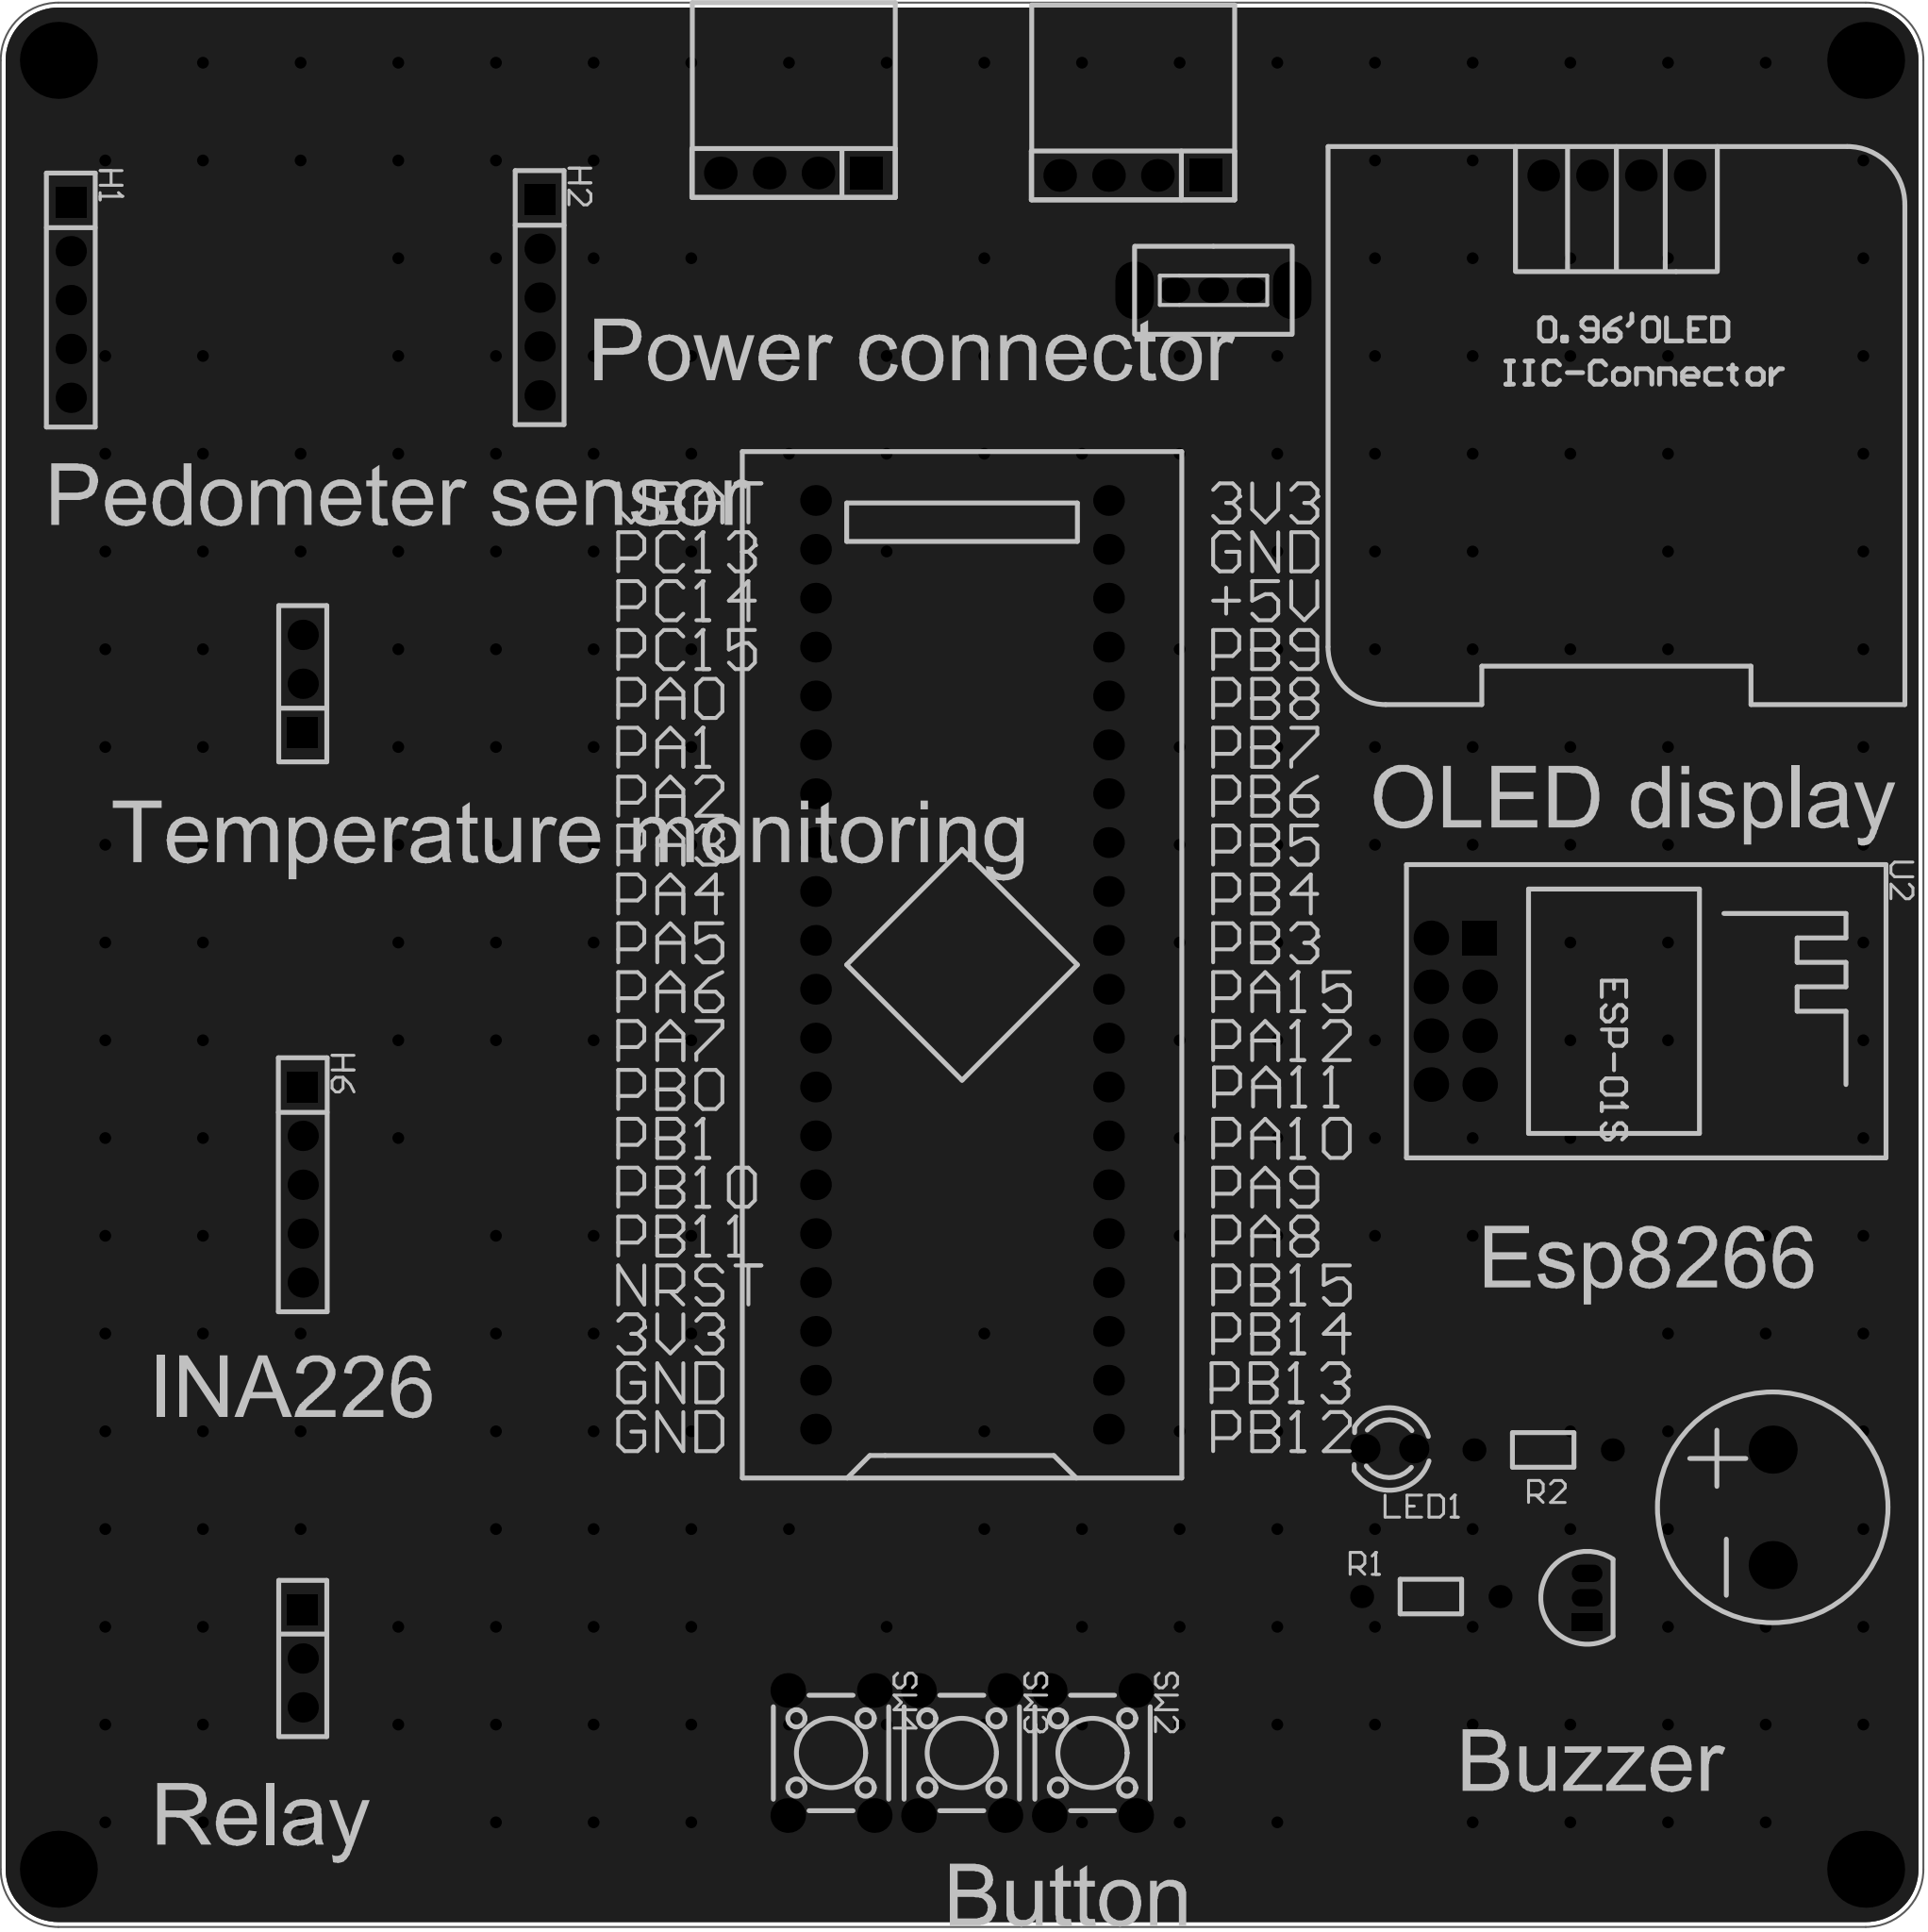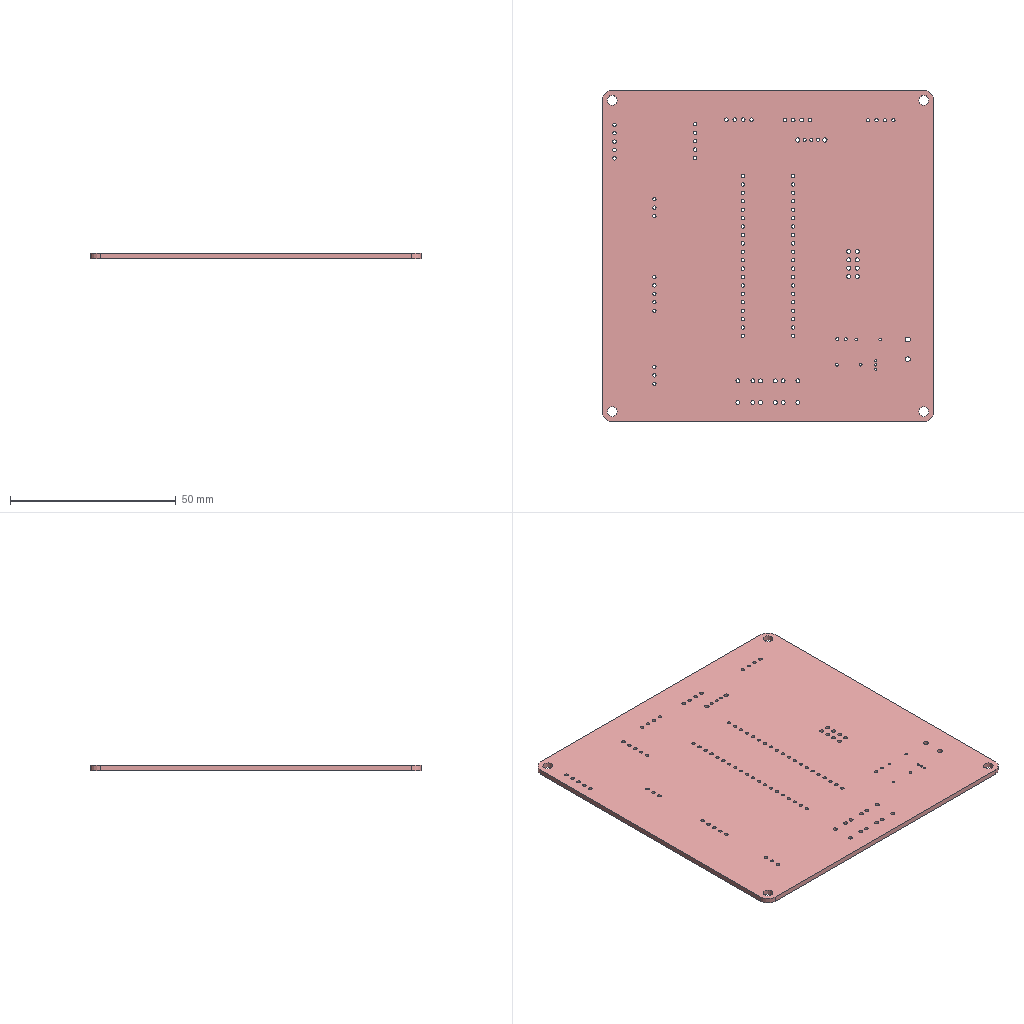Circuit board layout | Altium Designer | box 100 x 100 x 1.6 mm
Layer stack:
# Altium Designer layer stack of  (unit mm; dielectric type: 0 none, 1 core, 2 prepreg, 3 surface material)
index,name,kind,layer,copper_thickness_mm,dielectric_type,dielectric_thickness_mm,dielectric_material,dielectric_constant
0,Top Paste Mask Layer,other,,,,,,
1,Top Silkscreen Layer,other,,,,,,
2,Top Solder Mask Layer,dielectric,,,3,0.01,,3.3
3,Top Layer,copper,Top Layer,0.035,,,,
4,Dielectric1,dielectric,,,3,1.51,FR4,4.5
5,Bottom Layer,copper,Bottom Layer,0.035,,,,
6,Bottom Solder Mask Layer,dielectric,,,3,0.01,,3.3
7,Bottom Silkscreen Layer,other,,,,,,
8,Bottom Paste Mask Layer,other,,,,,,
# drill layer pairs: low layer,high layer
drill_pair,Top Layer,Bottom Layer
Part placement:
Designator,Comment,Layer,Footprint,Center-X(mm),Center-Y(mm),Rotation
U1,STM32F103C8T6-Card,TopLayer,CONN-TH_L53.3-W22.9_STM32F103C8T6-CARD,141.351,138.557,90
OLED1,,TopLayer,0.96OLED_4P,175.387,179.578,0
SW2,,TopLayer,SW-TH_4P-L6.0-W6.0-P4.50-LS6.5,148.136,97.599,270
SW3,,TopLayer,SW-TH_4P-L6.0-W6.0-P4.50-LS6.5,141.337,97.599,270
SW4,,TopLayer,SW-TH_4P-L6.0-W6.0-P4.50-LS6.5,134.537,97.599,270
H12,,TopLayer,HDR-TH_3P-P2.54-V-F,107.061,102.509,270
SW5,,TopLayer,拨动开关,154.424,173.609,180
H3,,TopLayer,HDR-TH_3P-P2.54-V-F,107.061,153.162,90
BUZZER1,buzzer,TopLayer,BUZ-TH_BD12.0-P6.00-D0.9-RD,183.515,110.363,90
Q1,,TopLayer,S8050_TO_92,173.863,105.664,90
H6,,TopLayer,HDR-TH_5P-P2.54-V-F,107.061,127.127,270
LED1,,TopLayer,LED_TH-3mm,163.576,113.411,180
R1,100Ω,TopLayer,Res_1/8W,165.735,105.727,0
R2,1kΩ,TopLayer,Res_1/8W,171.577,113.347,0
U2,ESP-01S,TopLayer,WIFIM-TH_ESP-01S,167.005,136.144,270
H1,,TopLayer,HDR-TH_5P-P2.54-V-F,94.996,173.101,270
H2,,TopLayer,HDR-TH_5P-P2.54-V-F,119.38,173.228,270
H4,,TopLayer,HDR-TH_4P-P2.54-V-F,132.588,179.705,180
H5,,TopLayer,HDR-TH_4P-P2.54-V-F,150.241,179.578,180
Pad and via stacks:
# Altium Designer via and pad stacks of  (unit mm). Each distinct definition once, with the count of objects using it.
# via: kind,start_layer,end_layer,hole_mm,diameter_mm,mode(0 simple;1 top-mid-bottom;2 full stack),diameter_per_layer,count,example_net
# pad: kind,layer,hole_mm,hole_type(0 round;1 square;2 slot),plating,top_size,top_shape(1 round;2 rect;3 octagon;9 rounded rect),mid_size,bottom_size,mode,footprint,size_per_layer,count,example
pad,Multi-Layer,3,0,plated,4x4,1,4x4,4x4,0,,,4,1
pad,Multi-Layer,1,0,plated,1.6x1.6,1,1.6x1.6,1.6x1.6,0,CONN-TH_L53.3-W22.9_STM32F103C8T6-CARD,,40,U1.1
pad,Multi-Layer,1,0,plated,1.65x1.65,1,1.65x1.65,1.65x1.65,0,0.96OLED_4P,,4,OLED1.4
pad,Multi-Layer,1.2,0,plated,1.8x1.8,1,1.8x1.8,1.8x1.8,0,SW-TH_4P-L6.0-W6.0-P4.50-LS6.5,,12,SW2.1
pad,Multi-Layer,1.02,0,plated,1.575x1.575,1,1.575x1.575,1.575x1.575,0,HDR-TH_3P-P2.54-V-F,,4,H12.3
pad,Multi-Layer,1.02,0,plated,1.575x1.575,2,1.575x1.575,1.575x1.575,0,HDR-TH_3P-P2.54-V-F,,2,H12.1
pad,Multi-Layer,0.8992,0,plated,1.6x1.3,1,1.6x1.3,1.6x1.3,0,\u00B2\u00A6\u00B6\u00AF\u00BF\u00AA\u00B9\u00D8,,3,SW5.1
pad,Multi-Layer,1.3,0,plated,3x1.999,1,3x1.999,3x1.999,0,\u00B2\u00A6\u00B6\u00AF\u00BF\u00AA\u00B9\u00D8,,2,SW5.4
pad,Multi-Layer,1.5,0,plated,2.5x2.5,1,2.5x2.5,2.5x2.5,0,BUZ-TH_BD12.0-P6.00-D0.9-RD,,2,BUZZER1.1
pad,Multi-Layer,0.701,0,plated,0.8992x1.6,2,0.8992x1.6,0.8992x1.6,0,S8050_TO_92,,1,Q1.1
pad,Multi-Layer,0.701,0,plated,0.8992x1.6,1,0.8992x1.6,0.8992x1.6,0,S8050_TO_92,,2,Q1.2
pad,Multi-Layer,1.02,0,plated,1.575x1.575,1,1.575x1.575,1.575x1.575,0,HDR-TH_5P-P2.54-V-F,,12,H6.5
pad,Multi-Layer,1.02,0,plated,1.575x1.575,2,1.575x1.575,1.575x1.575,0,HDR-TH_5P-P2.54-V-F,,3,H6.1
pad,Multi-Layer,0.9144,0,plated,1.524x1.524,1,1.524x1.524,1.524x1.524,0,LED_TH-3mm,,2,LED1.1
pad,Multi-Layer,0.8001,0,plated,1.199x1.199,1,1.199x1.199,1.199x1.199,0,Res_1/8W,,4,R1.1
pad,Multi-Layer,1.2,0,plated,1.8x1.8,2,1.8x1.8,1.8x1.8,0,WIFIM-TH_ESP-01S,,1,U2.1
pad,Multi-Layer,1.2,0,plated,1.8x1.8,1,1.8x1.8,1.8x1.8,0,WIFIM-TH_ESP-01S,,7,U2.2
pad,Multi-Layer,1.1,0,plated,1.7x1.7,2,1.7x1.7,1.7x1.7,0,HDR-TH_4P-P2.54-V-F,,2,H4.1
pad,Multi-Layer,1.1,0,plated,1.7x1.7,1,1.7x1.7,1.7x1.7,0,HDR-TH_4P-P2.54-V-F,,6,H4.2
via,Top Layer,Bottom Layer,0.3048,0.61,0,,249,GND
Copper pours:
name,layer,net,type(0 solid;1 hatched;2 none)
Bottom Layer-GND,Bottom Layer,GND,0
Bottom Layer-GND 1,Bottom Layer,GND,0
Top Layer-GND,Top Layer,GND,0